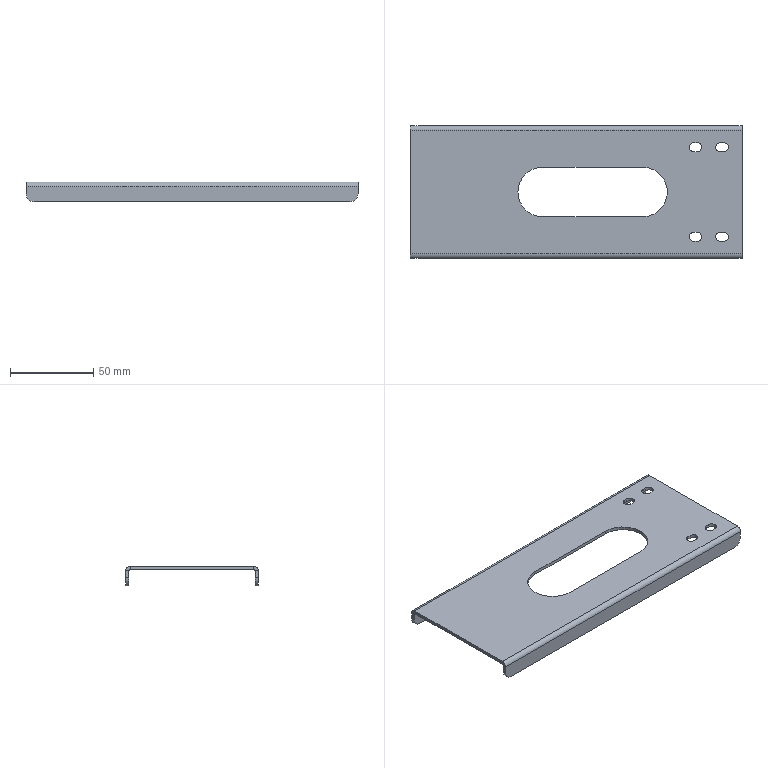Part | STEP file | B1-017 | 1 solid | 51 faces | box 200 x 80 x 12 mm | volume 34069 mm3 | plane 28 | cylinder 23 | commonest cylinder face diameters 5.5 x12 10 x4 30 x3 1.473 x2 5.473 x2